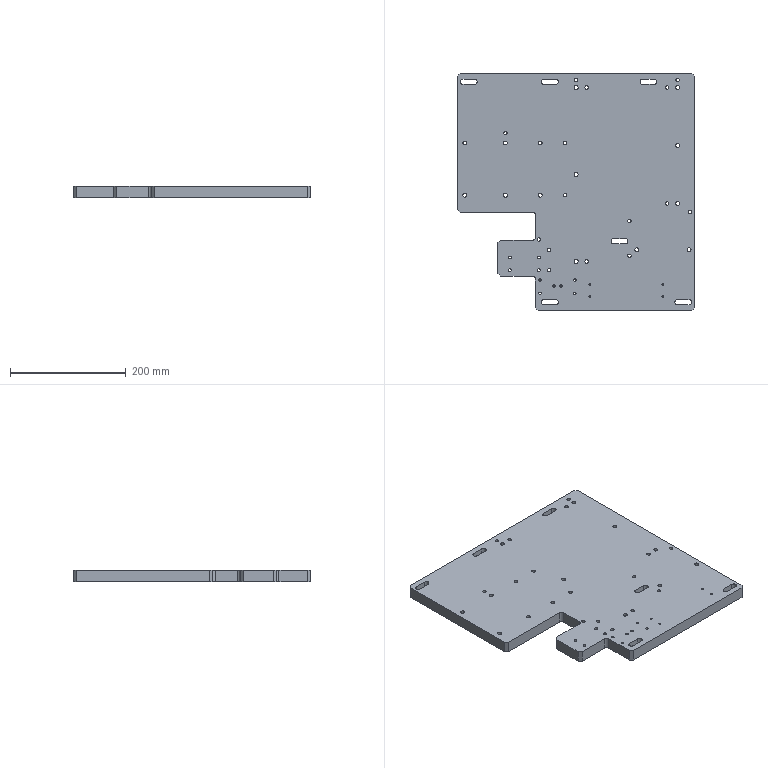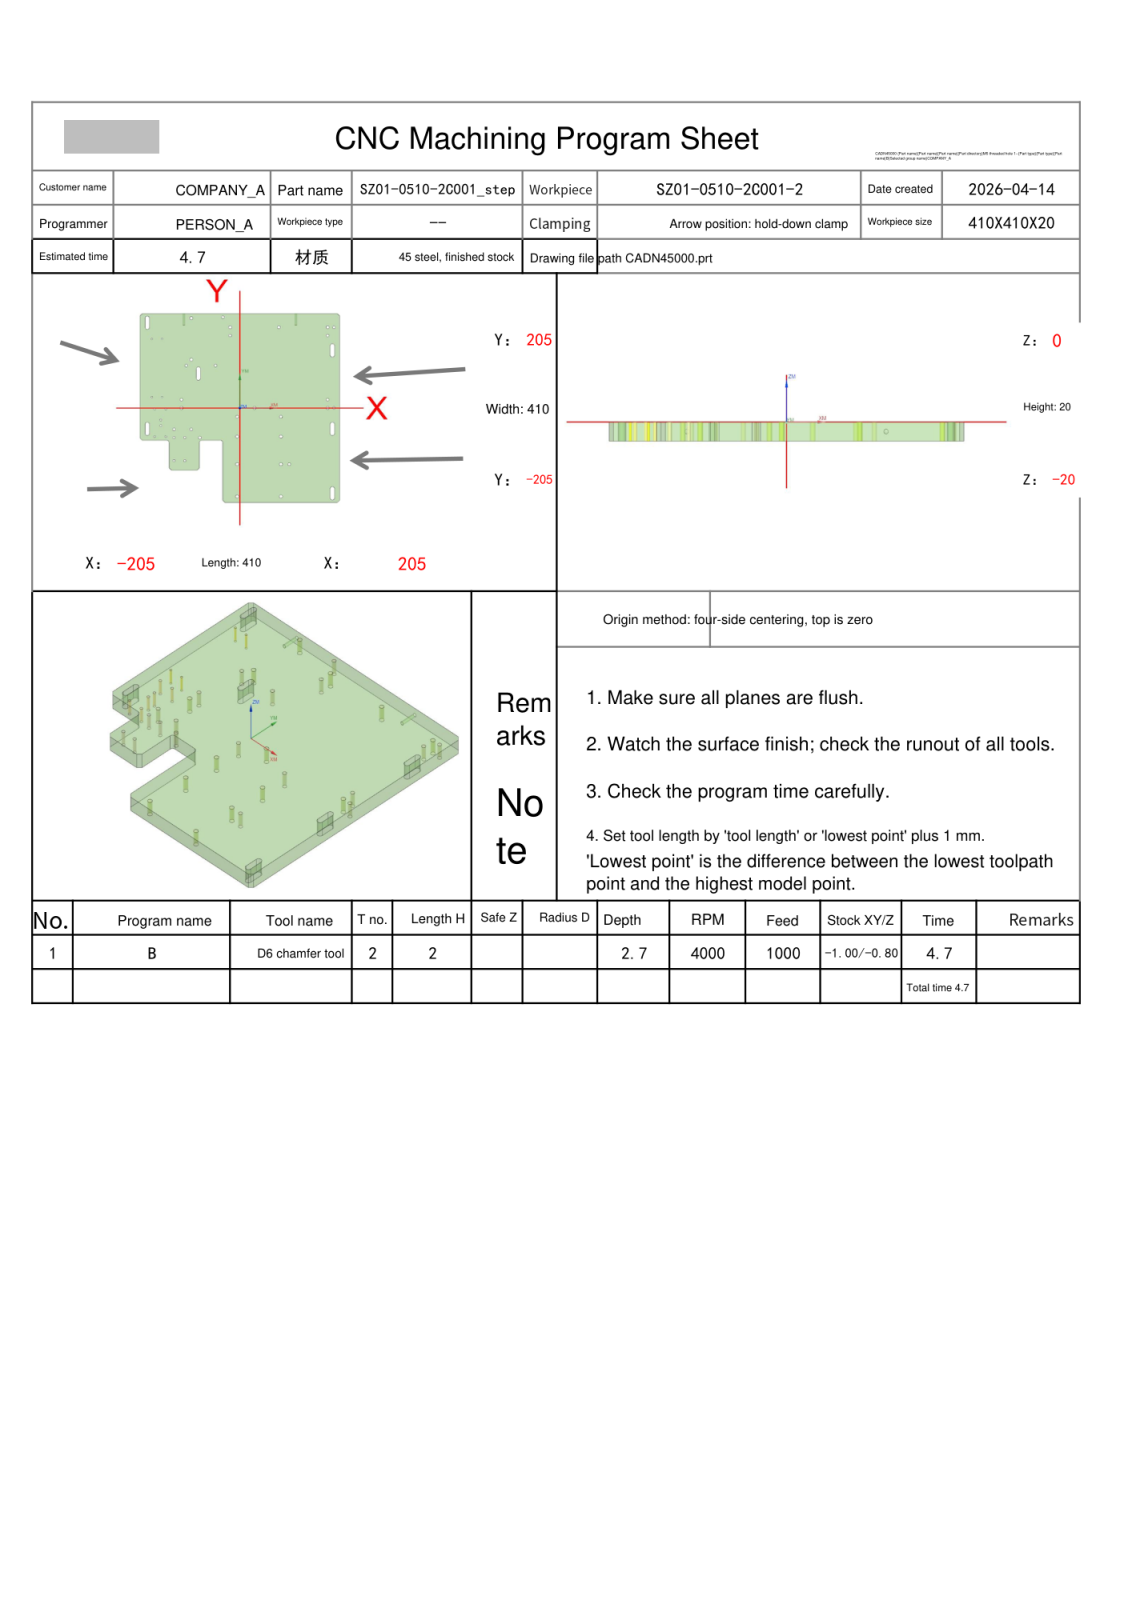NC program | NX | posted by the shop | part box 410 x 410 x 20 mm
Whole program:
%
O0001
(Machine time: 4.76 MIN)
(===Total Tool:1===)
(T2=D6 chamfer tool   D=6.   R=0.   D-  H02 Z=-2.7  )
G80 G90 G17 G49 G40
G91 G28 Z0
M01
N1 T02 M06
(D6 chamfer tool  D=6. R=0. H=02 ce=0.00 di=0.00)
G00 G90 G54 X-159.5 Y24. M03 S2000
G43 H02 Z50.
M08
G98 G81 X-159.5 Y24. Z-2.2 R3. F100.
X-180.5
Y150.
X-159.5
G80
G00 Z50.
G00 G90 X-175. Y-62. M03 S2000
Z50.
G98 G81 X-175. Y-62. Z-2.7 R3. F100.
X-152.
X-162.5 Y-37.96
Y-25.96
X-152. Y-2.
X-175.
G80
G00 Z50.
G00 G90 X-135.694 Y-64.308 M03 S4000
Z50.
Z-1.1
G01 Z-1.6 F300.
X-136.5 Y-64.415
G03 X-135. Y-65.915 I1.5 J0.0
X-133.3 Y-64.215 I0.0 J1.7
X-135. Y-62.515 I-1.7 J0.0
X-136.7 Y-64.215 I0.0 J-1.7
X-135. Y-65.915 I1.7 J0.0
X-133.5 Y-64.415 I0.0 J1.5
G01 X-134.306 Y-64.308
Z-1.1
G00 Z50.
X-113.694
Z-1.1
G01 Z-1.6
X-114.5 Y-64.415
G03 X-113. Y-65.915 I1.5 J0.0
X-111.3 Y-64.215 I0.0 J1.7
X-113. Y-62.515 I-1.7 J0.0
X-114.7 Y-64.215 I0.0 J-1.7
X-113. Y-65.915 I1.7 J0.0
X-111.5 Y-64.415 I0.0 J1.5
G01 X-112.306 Y-64.308
Z-1.1
G00 Z50.
X-113.694 Y-114.308
Z-1.1
G01 Z-1.6
X-114.5 Y-114.415
G03 X-113. Y-115.915 I1.5 J0.0
X-111.3 Y-114.215 I0.0 J1.7
X-113. Y-112.515 I-1.7 J0.0
X-114.7 Y-114.215 I0.0 J-1.7
X-113. Y-115.915 I1.7 J0.0
X-111.5 Y-114.415 I0.0 J1.5
G01 X-112.306 Y-114.308
Z-1.1
G00 Z50.
X-135.694
Z-1.1
G01 Z-1.6
X-136.5 Y-114.415
G03 X-135. Y-115.915 I1.5 J0.0
X-133.3 Y-114.215 I0.0 J1.7
X-135. Y-112.515 I-1.7 J0.0
X-136.7 Y-114.215 I0.0 J-1.7
X-135. Y-115.915 I1.7 J0.0
X-133.5 Y-114.415 I0.0 J1.5
G01 X-134.306 Y-114.308
Z-1.1
G00 Z50.
G00 G90 X-35.394 Y196.907 M03 S4000
Z50.
Z-1.1
G01 Z-1.6 F600.
X-36.2 Y196.8
G03 X-34.7 Y195.3 I1.5 J0.0
X-33. Y197. I0.0 J1.7
X-34.7 Y198.7 I-1.7 J0.0
X-36.4 Y197. I0.0 J-1.7
X-34.7 Y195.3 I1.7 J0.0
X-33.2 Y196.8 I0.0 J1.5
G01 X-34.006 Y196.907
Z-1.1
G00 Z50.
X-20.494 Y157.107
Z-1.1
G01 Z-1.6
X-21.3 Y157.
G03 X-19.8 Y155.5 I1.5 J0.0
X-18.1 Y157.2 I0.0 J1.7
X-19.8 Y158.9 I-1.7 J0.0
X-21.5 Y157.2 I0.0 J-1.7
X-19.8 Y155.5 I1.7 J0.0
X-18.3 Y157. I0.0 J1.5
G01 X-19.106 Y157.107
Z-1.1
G00 Z50.
X-50.694 Y91.907
Z-1.1
G01 Z-1.6
X-51.5 Y91.8
G03 X-50. Y90.3 I1.5 J0.0
X-48.3 Y92. I0.0 J1.7
X-50. Y93.7 I-1.7 J0.0
X-51.7 Y92. I0.0 J-1.7
X-50. Y90.3 I1.7 J0.0
X-48.5 Y91.8 I0.0 J1.5
G01 X-49.306 Y91.907
Z-1.1
G00 Z50.
X-110.694
Z-1.1
G01 Z-1.6
X-111.5 Y91.8
G03 X-110. Y90.3 I1.5 J0.0
X-108.3 Y92. I0.0 J1.7
X-110. Y93.7 I-1.7 J0.0
X-111.7 Y92. I0.0 J-1.7
X-110. Y90.3 I1.7 J0.0
X-108.5 Y91.8 I0.0 J1.5
G01 X-109.306 Y91.907
Z-1.1
G00 Z50.
X-120.494 Y18.107
Z-1.1
G01 Z-1.6
X-121.3 Y18.
G03 X-119.8 Y16.5 I1.5 J0.0
X-118.1 Y18.2 I0.0 J1.7
X-119.8 Y19.9 I-1.7 J0.0
X-121.5 Y18.2 I0.0 J-1.7
X-119.8 Y16.5 I1.7 J0.0
X-118.3 Y18. I0.0 J1.5
G01 X-119.106 Y18.107
Z-1.1
G00 Z50.
X-135.694 Y-46.308
Z-1.1
G01 Z-1.6
X-136.5 Y-46.415
G03 X-135. Y-47.915 I1.5 J0.0
X-133.3 Y-46.215 I0.0 J1.7
X-135. Y-44.515 I-1.7 J0.0
X-136.7 Y-46.215 I0.0 J-1.7
X-135. Y-47.915 I1.7 J0.0
X-133.5 Y-46.415 I0.0 J1.5
G01 X-134.306 Y-46.308
Z-1.1
G00 Z50.
X-100.694
Z-1.1
G01 Z-1.6
X-101.5 Y-46.415
G03 X-100. Y-47.915 I1.5 J0.0
X-98.3 Y-46.215 I0.0 J1.7
X-100. Y-44.515 I-1.7 J0.0
X-101.7 Y-46.215 I0.0 J-1.7
X-100. Y-47.915 I1.7 J0.0
X-98.5 Y-46.415 I0.0 J1.5
G01 X-99.306 Y-46.308
Z-1.1
G00 Z50.
X-82.694 Y-64.308
Z-1.1
G01 Z-1.6
X-83.5 Y-64.415
G03 X-82. Y-65.915 I1.5 J0.0
X-80.3 Y-64.215 I0.0 J1.7
X-82. Y-62.515 I-1.7 J0.0
X-83.7 Y-64.215 I0.0 J-1.7
X-82. Y-65.915 I1.7 J0.0
X-80.5 Y-64.415 I0.0 J1.5
G01 X-81.306 Y-64.308
Z-1.1
G00 Z50.
X-6.194 Y-18.943
Z-1.1
G01 Z-1.6
X-7. Y-19.05
G03 X-5.5 Y-20.55 I1.5 J0.0
X-3.8 Y-18.85 I0.0 J1.7
X-5.5 Y-17.15 I-1.7 J0.0
X-7.2 Y-18.85 I0.0 J-1.7
X-5.5 Y-20.55 I1.7 J0.0
X-4. Y-19.05 I0.0 J1.5
G01 X-4.806 Y-18.943
Z-1.1
G00 Z50.
X83.806
Z-1.1
G01 Z-1.6
X83. Y-19.05
G03 X84.5 Y-20.55 I1.5 J0.0
X86.2 Y-18.85 I0.0 J1.7
X84.5 Y-17.15 I-1.7 J0.0
X82.8 Y-18.85 I0.0 J-1.7
X84.5 Y-20.55 I1.7 J0.0
X86. Y-19.05 I0.0 J1.5
G01 X85.194 Y-18.943
Z-1.1
G00 Z50.
X100.776 Y-121.943
Z-1.1
G01 Z-1.6
X99.97 Y-122.05
G03 X101.47 Y-123.55 I1.5 J0.0
X103.17 Y-121.85 I0.0 J1.7
X101.47 Y-120.15 I-1.7 J0.0
X99.77 Y-121.85 I0.0 J-1.7
X101.47 Y-123.55 I1.7 J0.0
X102.97 Y-122.05 I0.0 J1.5
G01 X102.164 Y-121.943
Z-1.1
G00 Z50.
X192.506 Y.107
Z-1.1
G01 Z-1.6
X191.7 Y0.0
G03 X193.2 Y-1.5 I1.5 J0.0
X194.9 Y.2 I0.0 J1.7
X193.2 Y1.9 I-1.7 J0.0
X191.5 Y.2 I0.0 J-1.7
X193.2 Y-1.5 I1.7 J0.0
X194.7 Y0.0 I0.0 J1.5
G01 X193.894 Y.107
Z-1.1
G00 Z50.
X179.506 Y18.107
Z-1.1
G01 Z-1.6
X178.7 Y18.
G03 X180.2 Y16.5 I1.5 J0.0
X181.9 Y18.2 I0.0 J1.7
X180.2 Y19.9 I-1.7 J0.0
X178.5 Y18.2 I0.0 J-1.7
X180.2 Y16.5 I1.7 J0.0
X181.7 Y18. I0.0 J1.5
G01 X180.894 Y18.107
Z-1.1
G00 Z50.
X179.506 Y157.107
Z-1.1
G01 Z-1.6
X178.7 Y157.
G03 X180.2 Y155.5 I1.5 J0.0
X181.9 Y157.2 I0.0 J1.7
X180.2 Y158.9 I-1.7 J0.0
X178.5 Y157.2 I0.0 J-1.7
X180.2 Y155.5 I1.7 J0.0
X181.7 Y157. I0.0 J1.5
G01 X180.894 Y157.107
Z-1.1
G00 Z50.
X192.506 Y175.107
Z-1.1
G01 Z-1.6
X191.7 Y175.
G03 X193.2 Y173.5 I1.5 J0.0
X194.9 Y175.2 I0.0 J1.7
X193.2 Y176.9 I-1.7 J0.0
X191.5 Y175.2 I0.0 J-1.7
X193.2 Y173.5 I1.7 J0.0
X194.7 Y175. I0.0 J1.5
G01 X193.894 Y175.107
Z-1.1
G00 Z50.
G00 G90 X178.7 Y174.205 M03 S4000
Z50.
Z-1.1
G01 Z-1.6 F300.
Y173.9
G03 X180.2 Y172.4 I1.5 J0.0
X183. Y175.2 I0.0 J2.8
X180.2 Y178. I-2.8 J0.0
X177.4 Y175.2 I0.0 J-2.8
X180.2 Y172.4 I2.8 J0.0
X181.7 Y173.9 I0.0 J1.5
G01 Y174.205
Z-1.1
G00 Z50.
X78.7
Z-1.1
G01 Z-1.6
Y173.9
G03 X80.2 Y172.4 I1.5 J0.0
X83. Y175.2 I0.0 J2.8
X80.2 Y178. I-2.8 J0.0
X77.4 Y175.2 I0.0 J-2.8
X80.2 Y172.4 I2.8 J0.0
X81.7 Y173.9 I0.0 J1.5
G01 Y174.205
Z-1.1
G00 Z50.
X-21.3
Z-1.1
G01 Z-1.6
Y173.9
G03 X-19.8 Y172.4 I1.5 J0.0
X-17. Y175.2 I0.0 J2.8
X-19.8 Y178. I-2.8 J0.0
X-22.6 Y175.2 I0.0 J-2.8
X-19.8 Y172.4 I2.8 J0.0
X-18.3 Y173.9 I0.0 J1.5
G01 Y174.205
Z-1.1
G00 Z50.
X-101.245 Y194.005
Z-1.1
G01 Z-1.6
Y193.7
G03 X-99.745 Y192.2 I1.5 J0.0
X-96.945 Y195. I0.0 J2.8
X-99.745 Y197.8 I-2.8 J0.0
X-102.545 Y195. I0.0 J-2.8
X-99.745 Y192.2 I2.8 J0.0
X-98.245 Y193.7 I0.0 J1.5
G01 Y194.005
Z-1.1
G00 Z50.
X-101.245 Y104.005
Z-1.1
G01 Z-1.6
Y103.7
G03 X-99.745 Y102.2 I1.5 J0.0
X-96.945 Y105. I0.0 J2.8
X-99.745 Y107.8 I-2.8 J0.0
X-102.545 Y105. I0.0 J-2.8
X-99.745 Y102.2 I2.8 J0.0
X-98.245 Y103.7 I0.0 J1.5
G01 Y104.005
Z-1.1
G00 Z50.
X-121.3 Y-.795
Z-1.1
G01 Z-1.6
Y-1.1
G03 X-119.8 Y-2.6 I1.5 J0.0
X-117. Y.2 I0.0 J2.8
X-119.8 Y3. I-2.8 J0.0
X-122.6 Y.2 I0.0 J-2.8
X-119.8 Y-2.6 I2.8 J0.0
X-118.3 Y-1.1 I0.0 J1.5
G01 Y-.795
Z-1.1
G00 Z50.
X28.7
Z-1.1
G01 Z-1.6
Y-1.1
G03 X30.2 Y-2.6 I1.5 J0.0
X33. Y.2 I0.0 J2.8
X30.2 Y3. I-2.8 J0.0
X27.4 Y.2 I0.0 J-2.8
X30.2 Y-2.6 I2.8 J0.0
X31.7 Y-1.1 I0.0 J1.5
G01 Y-.795
Z-1.1
G00 Z50.
X-7. Y-62.845
Z-1.1
G01 Z-1.6
Y-63.15
G03 X-5.5 Y-64.65 I1.5 J0.0
X-2.7 Y-61.85 I0.0 J2.8
X-5.5 Y-59.05 I-2.8 J0.0
X-8.3 Y-61.85 I0.0 J-2.8
X-5.5 Y-64.65 I2.8 J0.0
X-4. Y-63.15 I0.0 J1.5
G01 Y-62.845
Z-1.1
G00 Z50.
X-7. Y-122.845
Z-1.1
G01 Z-1.6
Y-123.15
G03 X-5.5 Y-124.65 I1.5 J0.0
X-2.7 Y-121.85 I0.0 J2.8
X-5.5 Y-119.05 I-2.8 J0.0
X-8.3 Y-121.85 I0.0 J-2.8
X-5.5 Y-124.65 I2.8 J0.0
X-4. Y-123.15 I0.0 J1.5
G01 Y-122.845
Z-1.1
G00 Z50.
X-7. Y-192.845
Z-1.1
G01 Z-1.6
Y-193.15
G03 X-5.5 Y-194.65 I1.5 J0.0
X-2.7 Y-191.85 I0.0 J2.8
X-5.5 Y-189.05 I-2.8 J0.0
X-8.3 Y-191.85 I0.0 J-2.8
X-5.5 Y-194.65 I2.8 J0.0
X-4. Y-193.15 I0.0 J1.5
G01 Y-192.845
Z-1.1
G00 Z50.
X83.
Z-1.1
G01 Z-1.6
Y-193.15
G03 X84.5 Y-194.65 I1.5 J0.0
X87.3 Y-191.85 I0.0 J2.8
X84.5 Y-189.05 I-2.8 J0.0
X81.7 Y-191.85 I0.0 J-2.8
X84.5 Y-194.65 I2.8 J0.0
X86. Y-193.15 I0.0 J1.5
G01 Y-192.845
Z-1.1
G00 Z50.
X83. Y-122.845
Z-1.1
G01 Z-1.6
Y-123.15
G03 X84.5 Y-124.65 I1.5 J0.0
X87.3 Y-121.85 I0.0 J2.8
X84.5 Y-119.05 I-2.8 J0.0
X81.7 Y-121.85 I0.0 J-2.8
X84.5 Y-124.65 I2.8 J0.0
X86. Y-123.15 I0.0 J1.5
G01 Y-122.845
Z-1.1
G00 Z50.
X83. Y-62.845
Z-1.1
G01 Z-1.6
Y-63.15
G03 X84.5 Y-64.65 I1.5 J0.0
X87.3 Y-61.85 I0.0 J2.8
X84.5 Y-59.05 I-2.8 J0.0
X81.7 Y-61.85 I0.0 J-2.8
X84.5 Y-64.65 I2.8 J0.0
X86. Y-63.15 I0.0 J1.5
G01 Y-62.845
Z-1.1
G00 Z50.
X178.7 Y-.795
Z-1.1
G01 Z-1.6
Y-1.1
G03 X180.2 Y-2.6 I1.5 J0.0
X183. Y.2 I0.0 J2.8
X180.2 Y3. I-2.8 J0.0
X177.4 Y.2 I0.0 J-2.8
X180.2 Y-2.6 I2.8 J0.0
X181.7 Y-1.1 I0.0 J1.5
G01 Y-.795
Z-1.1
G00 Z50.
G00 G90 X186.4 Y-184.834 M03 S4000
Z50.
Z2.5
G01 Y-195. Z-1.2 F1000.
G03 X190. Y-198.6 I3.6 J0.0
X193.6 Y-195. I0.0 J3.6
G01 Y-175.
G03 X190. Y-171.4 I-3.6 J0.0
X186.4 Y-175. I0.0 J-3.6
G01 Y-195.
G03 X186.435 Y-195.498 I3.6 J0.0
G01 Z1.3
G00 Z50.
X186.4 Y-44.834
Z2.5
G01 Y-55. Z-1.2
G03 X190. Y-58.6 I3.6 J0.0
X193.6 Y-55. I0.0 J3.6
G01 Y-35.
G03 X190. Y-31.4 I-3.6 J0.0
X186.4 Y-35. I0.0 J-3.6
G01 Y-55.
G03 X186.435 Y-55.498 I3.6 J0.0
G01 Z1.3
G00 Z50.
X186.4 Y125.166
Z2.5
G01 Y115. Z-1.2
G03 X190. Y111.4 I3.6 J0.0
X193.6 Y115. I0.0 J3.6
G01 Y135.
G03 X190. Y138.6 I-3.6 J0.0
X186.4 Y135. I0.0 J-3.6
G01 Y115.
G03 X186.435 Y114.502 I3.6 J0.0
G01 Z1.3
G00 Z50.
X-88.6 Y75.166
Z2.5
G01 Y65. Z-1.2
G03 X-85. Y61.4 I3.6 J0.0
X-81.4 Y65. I0.0 J3.6
G01 Y85.
G03 X-85. Y88.6 I-3.6 J0.0
X-88.6 Y85. I0.0 J-3.6
G01 Y65.
G03 X-88.565 Y64.502 I3.6 J0.0
G01 Z1.3
G00 Z50.
X-193.6 Y185.166
Z2.5
G01 Y175. Z-1.2
G03 X-190. Y171.4 I3.6 J0.0
X-186.4 Y175. I0.0 J3.6
G01 Y195.
G03 X-190. Y198.6 I-3.6 J0.0
X-193.6 Y195. I0.0 J-3.6
G01 Y175.
G03 X-193.565 Y174.502 I3.6 J0.0
G01 Z1.3
G00 Z50.
X-193.6 Y-44.834
Z2.5
G01 Y-55. Z-1.2
G03 X-190. Y-58.6 I3.6 J0.0
X-186.4 Y-55. I0.0 J3.6
G01 Y-35.
G03 X-190. Y-31.4 I-3.6 J0.0
X-193.6 Y-35. I0.0 J-3.6
G01 Y-55.
G03 X-193.565 Y-55.498 I3.6 J0.0
G01 Z1.3
G00 Z50.
G00 G90 X197.012 Y-206.2 M03 S4000
Z50.
Z2.5
G01 X199.876 Z1.458 F1000.
X199.971 Z1.423
X200.215 Y-206.164 Z1.333
X200.451 Y-206.089 Z1.243
X200.671 Y-205.975 Z1.153
X200.869 Y-205.828 Z1.063
X200.936 Y-205.761 Z1.028
X205.849 Y-200.849 Z-1.5
X200.936 Y-205.761
G02 X199.876 Y-206.2 I-1.061 J1.061
G01 X-29.876
G02 X-30.936 Y-205.761 I0.0 J1.5
G01 X-35.761 Y-200.936
G02 X-36.2 Y-199.876 I1.061 J1.061
G01 Y-75.
G03 X-40. Y-71.2 I-3.8 J0.0
G01 X-78.
G03 X-81.8 Y-75. I0.0 J-3.8
G01 Y-129.876
G02 X-82.239 Y-130.936 I-1.5 J0.0
G01 X-87.064 Y-135.761
G02 X-88.124 Y-136.2 I-1.061 J1.061
G01 X-139.876
G02 X-140.936 Y-135.761 I0.0 J1.5
G01 X-145.761 Y-130.936
G02 X-146.2 Y-129.876 I1.061 J1.061
G01 Y-75.
G03 X-150. Y-71.2 I-3.8 J0.0
G01 X-199.876
G02 X-200.936 Y-70.761 I0.0 J1.5
G01 X-205.849 Y-65.849
Z1.
G00 Z50.
X-197.012 Y206.2
Z2.5
G01 X-199.876 Z1.458
X-199.971 Z1.423
X-200.215 Y206.164 Z1.333
X-200.451 Y206.089 Z1.243
X-200.671 Y205.975 Z1.153
X-200.869 Y205.828 Z1.063
X-205.849 Y200.849 Z-1.5
X-200.936 Y205.761
G02 X-199.876 Y206.2 I1.061 J-1.061
G01 X199.876
G02 X200.936 Y205.761 I0.0 J-1.5
G01 X205.849 Y200.849
Z1.
G00 Z50.
M05
M09
G91 G28 Z0.0
G91 G28 Y0.0
M30
%